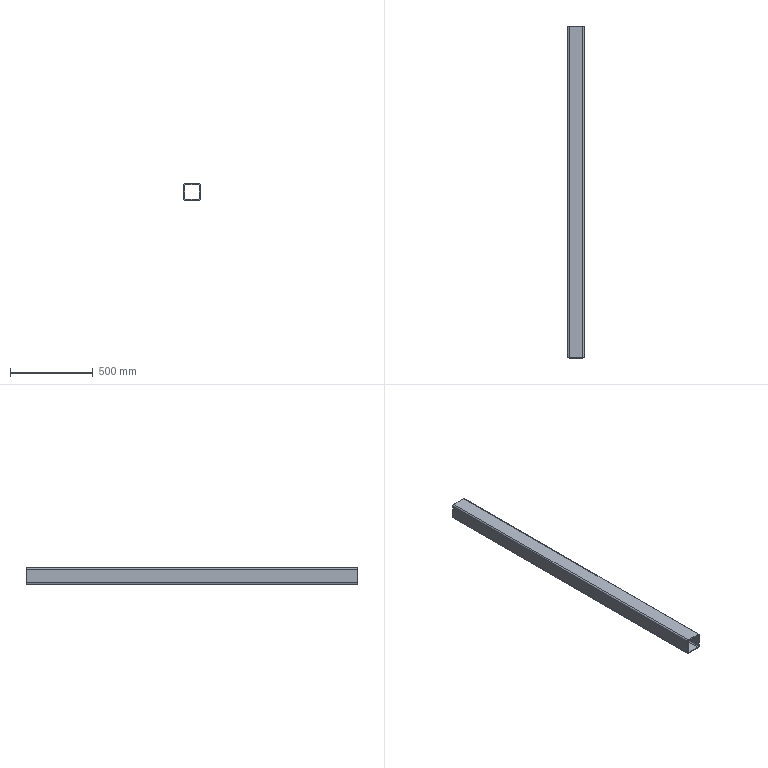Part | SolidWorks | features Extrusion 1 | 1 solid | 18 faces | box 100 x 2000 x 100 mm | volume 4684151 mm3 | plane 10 | cylinder 8 | commonest cylinder face diameters 12.6 x4 15.75 x4
STEP:
#1=CARTESIAN_POINT('',(100.,1000.,-90.6));
#2=VERTEX_POINT('',#1);
#3=CARTESIAN_POINT('',(92.125,1000.,-98.475));
#4=VERTEX_POINT('',#3);
#5=CARTESIAN_POINT('',(92.125,1000.,-90.6));
#6=DIRECTION('',(0.,1.,0.));
#7=DIRECTION('',(0.,0.,1.));
#8=AXIS2_PLACEMENT_3D('',#5,#6,#7);
#9=CIRCLE('',#8,7.875);
#10=EDGE_CURVE('',#2,#4,#9,.T.);
#11=ORIENTED_EDGE('',*,*,#10,.T.);
#12=CARTESIAN_POINT('',(7.875,1000.,-98.475));
#13=VERTEX_POINT('',#12);
#14=CARTESIAN_POINT('',(92.125,1000.,-98.475));
#15=DIRECTION('',(-1.,0.,0.));
#16=VECTOR('',#15,1000.);
#17=LINE('',#14,#16);
#18=EDGE_CURVE('',#4,#13,#17,.T.);
#19=ORIENTED_EDGE('',*,*,#18,.T.);
#20=CARTESIAN_POINT('',(0.,1000.,-90.6));
#21=VERTEX_POINT('',#20);
#22=CARTESIAN_POINT('',(7.875,1000.,-90.6));
#23=DIRECTION('',(0.,1.,0.));
#24=DIRECTION('',(0.,0.,1.));
#25=AXIS2_PLACEMENT_3D('',#22,#23,#24);
#26=CIRCLE('',#25,7.875);
#27=EDGE_CURVE('',#13,#21,#26,.T.);
#28=ORIENTED_EDGE('',*,*,#27,.T.);
#29=CARTESIAN_POINT('',(0.,1000.,-6.35));
#30=VERTEX_POINT('',#29);
#31=CARTESIAN_POINT('',(0.,1000.,-6.35));
#32=DIRECTION('',(0.,0.,1.));
#33=VECTOR('',#32,1000.);
#34=LINE('',#31,#33);
#35=EDGE_CURVE('',#21,#30,#34,.T.);
#36=ORIENTED_EDGE('',*,*,#35,.T.);
#37=CARTESIAN_POINT('',(7.875,1000.,1.525));
#38=VERTEX_POINT('',#37);
#39=CARTESIAN_POINT('',(7.875,1000.,-6.35));
#40=DIRECTION('',(0.,1.,0.));
#41=DIRECTION('',(0.,0.,1.));
#42=AXIS2_PLACEMENT_3D('',#39,#40,#41);
#43=CIRCLE('',#42,7.875);
#44=EDGE_CURVE('',#30,#38,#43,.T.);
#45=ORIENTED_EDGE('',*,*,#44,.T.);
#46=CARTESIAN_POINT('',(92.125,1000.,1.525));
#47=VERTEX_POINT('',#46);
#48=CARTESIAN_POINT('',(7.875,1000.,1.525));
#49=DIRECTION('',(1.,0.,0.));
#50=VECTOR('',#49,1000.);
#51=LINE('',#48,#50);
#52=EDGE_CURVE('',#38,#47,#51,.T.);
#53=ORIENTED_EDGE('',*,*,#52,.T.);
#54=CARTESIAN_POINT('',(100.,1000.,-6.35));
#55=VERTEX_POINT('',#54);
#56=CARTESIAN_POINT('',(92.125,1000.,-6.35));
#57=DIRECTION('',(0.,1.,0.));
#58=DIRECTION('',(0.,0.,1.));
#59=AXIS2_PLACEMENT_3D('',#56,#57,#58);
#60=CIRCLE('',#59,7.875);
#61=EDGE_CURVE('',#47,#55,#60,.T.);
#62=ORIENTED_EDGE('',*,*,#61,.T.);
#63=CARTESIAN_POINT('',(100.,1000.,-90.6));
#64=DIRECTION('',(0.,0.,-1.));
#65=VECTOR('',#64,1000.);
#66=LINE('',#63,#65);
#67=EDGE_CURVE('',#55,#2,#66,.T.);
#68=ORIENTED_EDGE('',*,*,#67,.T.);
#69=EDGE_LOOP('',(#11,#19,#28,#36,#45,#53,#62,#68));
#70=FACE_OUTER_BOUND('',#69,.T.);
#71=CARTESIAN_POINT('',(6.3,1000.,-85.875));
#72=VERTEX_POINT('',#71);
#73=CARTESIAN_POINT('',(6.3,1000.,-11.075));
#74=VERTEX_POINT('',#73);
#75=CARTESIAN_POINT('',(6.3,1000.,-11.075));
#76=DIRECTION('',(0.,0.,1.));
#77=VECTOR('',#76,1000.);
#78=LINE('',#75,#77);
#79=EDGE_CURVE('',#72,#74,#78,.T.);
#80=ORIENTED_EDGE('',*,*,#79,.F.);
#81=CARTESIAN_POINT('',(12.6,1000.,-92.175));
#82=VERTEX_POINT('',#81);
#83=CARTESIAN_POINT('',(12.6,1000.,-85.875));
#84=DIRECTION('',(0.,1.,0.));
#85=DIRECTION('',(0.,0.,1.));
#86=AXIS2_PLACEMENT_3D('',#83,#84,#85);
#87=CIRCLE('',#86,6.3);
#88=EDGE_CURVE('',#82,#72,#87,.T.);
#89=ORIENTED_EDGE('',*,*,#88,.F.);
#90=CARTESIAN_POINT('',(87.4,1000.,-92.175));
#91=VERTEX_POINT('',#90);
#92=CARTESIAN_POINT('',(87.4,1000.,-92.175));
#93=DIRECTION('',(-1.,0.,0.));
#94=VECTOR('',#93,1000.);
#95=LINE('',#92,#94);
#96=EDGE_CURVE('',#91,#82,#95,.T.);
#97=ORIENTED_EDGE('',*,*,#96,.F.);
#98=CARTESIAN_POINT('',(93.7,1000.,-85.875));
#99=VERTEX_POINT('',#98);
#100=CARTESIAN_POINT('',(87.4,1000.,-85.875));
#101=DIRECTION('',(0.,1.,0.));
#102=DIRECTION('',(0.,0.,1.));
#103=AXIS2_PLACEMENT_3D('',#100,#101,#102);
#104=CIRCLE('',#103,6.3);
#105=EDGE_CURVE('',#99,#91,#104,.T.);
#106=ORIENTED_EDGE('',*,*,#105,.F.);
#107=CARTESIAN_POINT('',(93.7,1000.,-11.075));
#108=VERTEX_POINT('',#107);
#109=CARTESIAN_POINT('',(93.7,1000.,-85.875));
#110=DIRECTION('',(0.,0.,-1.));
#111=VECTOR('',#110,1000.);
#112=LINE('',#109,#111);
#113=EDGE_CURVE('',#108,#99,#112,.T.);
#114=ORIENTED_EDGE('',*,*,#113,.F.);
#115=CARTESIAN_POINT('',(87.4,1000.,-4.775));
#116=VERTEX_POINT('',#115);
#117=CARTESIAN_POINT('',(87.4,1000.,-11.075));
#118=DIRECTION('',(0.,1.,0.));
#119=DIRECTION('',(0.,0.,1.));
#120=AXIS2_PLACEMENT_3D('',#117,#118,#119);
#121=CIRCLE('',#120,6.3);
#122=EDGE_CURVE('',#116,#108,#121,.T.);
#123=ORIENTED_EDGE('',*,*,#122,.F.);
#124=CARTESIAN_POINT('',(12.6,1000.,-4.775));
#125=VERTEX_POINT('',#124);
#126=CARTESIAN_POINT('',(12.6,1000.,-4.775));
#127=DIRECTION('',(1.,0.,0.));
#128=VECTOR('',#127,1000.);
#129=LINE('',#126,#128);
#130=EDGE_CURVE('',#125,#116,#129,.T.);
#131=ORIENTED_EDGE('',*,*,#130,.F.);
#132=CARTESIAN_POINT('',(12.6,1000.,-11.075));
#133=DIRECTION('',(0.,1.,0.));
#134=DIRECTION('',(0.,0.,1.));
#135=AXIS2_PLACEMENT_3D('',#132,#133,#134);
#136=CIRCLE('',#135,6.3);
#137=EDGE_CURVE('',#74,#125,#136,.T.);
#138=ORIENTED_EDGE('',*,*,#137,.F.);
#139=EDGE_LOOP('',(#80,#89,#97,#106,#114,#123,#131,#138));
#140=FACE_BOUND('',#139,.T.);
#141=CARTESIAN_POINT('',(92.125,1000.,-90.6));
#142=DIRECTION('',(0.,1.,0.));
#143=DIRECTION('',(0.,0.,1.));
#144=AXIS2_PLACEMENT_3D('',#141,#142,#143);
#145=PLANE('',#144);
#146=ADVANCED_FACE('',(#70,#140),#145,.T.);
#147=CARTESIAN_POINT('',(100.,-1000.,-90.6));
#148=VERTEX_POINT('',#147);
#149=CARTESIAN_POINT('',(92.125,-1000.,-98.475));
#150=VERTEX_POINT('',#149);
#151=CARTESIAN_POINT('',(92.125,-1000.,-90.6));
#152=DIRECTION('',(0.,1.,0.));
#153=DIRECTION('',(0.,0.,1.));
#154=AXIS2_PLACEMENT_3D('',#151,#152,#153);
#155=CIRCLE('',#154,7.875);
#156=EDGE_CURVE('',#148,#150,#155,.T.);
#157=ORIENTED_EDGE('',*,*,#156,.F.);
#158=CARTESIAN_POINT('',(100.,-1000.,-6.35));
#159=VERTEX_POINT('',#158);
#160=CARTESIAN_POINT('',(100.,-1000.,-90.6));
#161=DIRECTION('',(0.,0.,-1.));
#162=VECTOR('',#161,1000.);
#163=LINE('',#160,#162);
#164=EDGE_CURVE('',#159,#148,#163,.T.);
#165=ORIENTED_EDGE('',*,*,#164,.F.);
#166=CARTESIAN_POINT('',(92.125,-1000.,1.525));
#167=VERTEX_POINT('',#166);
#168=CARTESIAN_POINT('',(92.125,-1000.,-6.35));
#169=DIRECTION('',(0.,1.,0.));
#170=DIRECTION('',(0.,0.,1.));
#171=AXIS2_PLACEMENT_3D('',#168,#169,#170);
#172=CIRCLE('',#171,7.875);
#173=EDGE_CURVE('',#167,#159,#172,.T.);
#174=ORIENTED_EDGE('',*,*,#173,.F.);
#175=CARTESIAN_POINT('',(7.875,-1000.,1.525));
#176=VERTEX_POINT('',#175);
#177=CARTESIAN_POINT('',(7.875,-1000.,1.525));
#178=DIRECTION('',(1.,0.,0.));
#179=VECTOR('',#178,1000.);
#180=LINE('',#177,#179);
#181=EDGE_CURVE('',#176,#167,#180,.T.);
#182=ORIENTED_EDGE('',*,*,#181,.F.);
#183=CARTESIAN_POINT('',(0.,-1000.,-6.35));
#184=VERTEX_POINT('',#183);
#185=CARTESIAN_POINT('',(7.875,-1000.,-6.35));
#186=DIRECTION('',(0.,1.,0.));
#187=DIRECTION('',(0.,0.,1.));
#188=AXIS2_PLACEMENT_3D('',#185,#186,#187);
#189=CIRCLE('',#188,7.875);
#190=EDGE_CURVE('',#184,#176,#189,.T.);
#191=ORIENTED_EDGE('',*,*,#190,.F.);
#192=CARTESIAN_POINT('',(0.,-1000.,-90.6));
#193=VERTEX_POINT('',#192);
#194=CARTESIAN_POINT('',(0.,-1000.,-6.35));
#195=DIRECTION('',(0.,0.,1.));
#196=VECTOR('',#195,1000.);
#197=LINE('',#194,#196);
#198=EDGE_CURVE('',#193,#184,#197,.T.);
#199=ORIENTED_EDGE('',*,*,#198,.F.);
#200=CARTESIAN_POINT('',(7.875,-1000.,-98.475));
#201=VERTEX_POINT('',#200);
#202=CARTESIAN_POINT('',(7.875,-1000.,-90.6));
#203=DIRECTION('',(0.,1.,0.));
#204=DIRECTION('',(0.,0.,1.));
#205=AXIS2_PLACEMENT_3D('',#202,#203,#204);
#206=CIRCLE('',#205,7.875);
#207=EDGE_CURVE('',#201,#193,#206,.T.);
#208=ORIENTED_EDGE('',*,*,#207,.F.);
#209=CARTESIAN_POINT('',(92.125,-1000.,-98.475));
#210=DIRECTION('',(-1.,0.,0.));
#211=VECTOR('',#210,1000.);
#212=LINE('',#209,#211);
#213=EDGE_CURVE('',#150,#201,#212,.T.);
#214=ORIENTED_EDGE('',*,*,#213,.F.);
#215=EDGE_LOOP('',(#157,#165,#174,#182,#191,#199,#208,#214));
#216=FACE_OUTER_BOUND('',#215,.T.);
#217=CARTESIAN_POINT('',(12.6,-1000.,-92.175));
#218=VERTEX_POINT('',#217);
#219=CARTESIAN_POINT('',(6.3,-1000.,-85.875));
#220=VERTEX_POINT('',#219);
#221=CARTESIAN_POINT('',(12.6,-1000.,-85.875));
#222=DIRECTION('',(0.,1.,0.));
#223=DIRECTION('',(0.,0.,1.));
#224=AXIS2_PLACEMENT_3D('',#221,#222,#223);
#225=CIRCLE('',#224,6.3);
#226=EDGE_CURVE('',#218,#220,#225,.T.);
#227=ORIENTED_EDGE('',*,*,#226,.T.);
#228=CARTESIAN_POINT('',(6.3,-1000.,-11.075));
#229=VERTEX_POINT('',#228);
#230=CARTESIAN_POINT('',(6.3,-1000.,-11.075));
#231=DIRECTION('',(0.,0.,1.));
#232=VECTOR('',#231,1000.);
#233=LINE('',#230,#232);
#234=EDGE_CURVE('',#220,#229,#233,.T.);
#235=ORIENTED_EDGE('',*,*,#234,.T.);
#236=CARTESIAN_POINT('',(12.6,-1000.,-4.775));
#237=VERTEX_POINT('',#236);
#238=CARTESIAN_POINT('',(12.6,-1000.,-11.075));
#239=DIRECTION('',(0.,1.,0.));
#240=DIRECTION('',(0.,0.,1.));
#241=AXIS2_PLACEMENT_3D('',#238,#239,#240);
#242=CIRCLE('',#241,6.3);
#243=EDGE_CURVE('',#229,#237,#242,.T.);
#244=ORIENTED_EDGE('',*,*,#243,.T.);
#245=CARTESIAN_POINT('',(87.4,-1000.,-4.775));
#246=VERTEX_POINT('',#245);
#247=CARTESIAN_POINT('',(12.6,-1000.,-4.775));
#248=DIRECTION('',(1.,0.,0.));
#249=VECTOR('',#248,1000.);
#250=LINE('',#247,#249);
#251=EDGE_CURVE('',#237,#246,#250,.T.);
#252=ORIENTED_EDGE('',*,*,#251,.T.);
#253=CARTESIAN_POINT('',(93.7,-1000.,-11.075));
#254=VERTEX_POINT('',#253);
#255=CARTESIAN_POINT('',(87.4,-1000.,-11.075));
#256=DIRECTION('',(0.,1.,0.));
#257=DIRECTION('',(0.,0.,1.));
#258=AXIS2_PLACEMENT_3D('',#255,#256,#257);
#259=CIRCLE('',#258,6.3);
#260=EDGE_CURVE('',#246,#254,#259,.T.);
#261=ORIENTED_EDGE('',*,*,#260,.T.);
#262=CARTESIAN_POINT('',(93.7,-1000.,-85.875));
#263=VERTEX_POINT('',#262);
#264=CARTESIAN_POINT('',(93.7,-1000.,-85.875));
#265=DIRECTION('',(0.,0.,-1.));
#266=VECTOR('',#265,1000.);
#267=LINE('',#264,#266);
#268=EDGE_CURVE('',#254,#263,#267,.T.);
#269=ORIENTED_EDGE('',*,*,#268,.T.);
#270=CARTESIAN_POINT('',(87.4,-1000.,-92.175));
#271=VERTEX_POINT('',#270);
#272=CARTESIAN_POINT('',(87.4,-1000.,-85.875));
#273=DIRECTION('',(0.,1.,0.));
#274=DIRECTION('',(0.,0.,1.));
#275=AXIS2_PLACEMENT_3D('',#272,#273,#274);
#276=CIRCLE('',#275,6.3);
#277=EDGE_CURVE('',#263,#271,#276,.T.);
#278=ORIENTED_EDGE('',*,*,#277,.T.);
#279=CARTESIAN_POINT('',(87.4,-1000.,-92.175));
#280=DIRECTION('',(-1.,0.,0.));
#281=VECTOR('',#280,1000.);
#282=LINE('',#279,#281);
#283=EDGE_CURVE('',#271,#218,#282,.T.);
#284=ORIENTED_EDGE('',*,*,#283,.T.);
#285=EDGE_LOOP('',(#227,#235,#244,#252,#261,#269,#278,#284));
#286=FACE_BOUND('',#285,.T.);
#287=CARTESIAN_POINT('',(92.125,-1000.,-90.6));
#288=DIRECTION('',(0.,1.,0.));
#289=DIRECTION('',(0.,0.,1.));
#290=AXIS2_PLACEMENT_3D('',#287,#288,#289);
#291=PLANE('',#290);
#292=ADVANCED_FACE('',(#216,#286),#291,.F.);
#293=ORIENTED_EDGE('',*,*,#156,.T.);
#294=CARTESIAN_POINT('',(92.125,1000.,-98.475));
#295=DIRECTION('',(0.,-1.,0.));
#296=VECTOR('',#295,1000.);
#297=LINE('',#294,#296);
#298=EDGE_CURVE('',#4,#150,#297,.T.);
#299=ORIENTED_EDGE('',*,*,#298,.F.);
#300=ORIENTED_EDGE('',*,*,#10,.F.);
#301=CARTESIAN_POINT('',(100.,1000.,-90.6));
#302=DIRECTION('',(0.,-1.,0.));
#303=VECTOR('',#302,1000.);
#304=LINE('',#301,#303);
#305=EDGE_CURVE('',#2,#148,#304,.T.);
#306=ORIENTED_EDGE('',*,*,#305,.T.);
#307=EDGE_LOOP('',(#293,#299,#300,#306));
#308=FACE_OUTER_BOUND('',#307,.T.);
#309=CARTESIAN_POINT('',(92.125,1000.,-90.6));
#310=DIRECTION('',(0.,-1.,0.));
#311=DIRECTION('',(0.,0.,-1.));
#312=AXIS2_PLACEMENT_3D('',#309,#310,#311);
#313=CYLINDRICAL_SURFACE('',#312,7.875);
#314=ADVANCED_FACE('',(#308),#313,.T.);
#315=ORIENTED_EDGE('',*,*,#213,.T.);
#316=CARTESIAN_POINT('',(7.875,1000.,-98.475));
#317=DIRECTION('',(0.,-1.,0.));
#318=VECTOR('',#317,1000.);
#319=LINE('',#316,#318);
#320=EDGE_CURVE('',#13,#201,#319,.T.);
#321=ORIENTED_EDGE('',*,*,#320,.F.);
#322=ORIENTED_EDGE('',*,*,#18,.F.);
#323=ORIENTED_EDGE('',*,*,#298,.T.);
#324=EDGE_LOOP('',(#315,#321,#322,#323));
#325=FACE_OUTER_BOUND('',#324,.T.);
#326=CARTESIAN_POINT('',(92.125,1000.,-98.475));
#327=DIRECTION('',(0.,0.,1.));
#328=DIRECTION('',(1.,0.,0.));
#329=AXIS2_PLACEMENT_3D('',#326,#327,#328);
#330=PLANE('',#329);
#331=ADVANCED_FACE('',(#325),#330,.F.);
#332=ORIENTED_EDGE('',*,*,#207,.T.);
#333=CARTESIAN_POINT('',(0.,1000.,-90.6));
#334=DIRECTION('',(0.,-1.,0.));
#335=VECTOR('',#334,1000.);
#336=LINE('',#333,#335);
#337=EDGE_CURVE('',#21,#193,#336,.T.);
#338=ORIENTED_EDGE('',*,*,#337,.F.);
#339=ORIENTED_EDGE('',*,*,#27,.F.);
#340=ORIENTED_EDGE('',*,*,#320,.T.);
#341=EDGE_LOOP('',(#332,#338,#339,#340));
#342=FACE_OUTER_BOUND('',#341,.T.);
#343=CARTESIAN_POINT('',(7.875,1000.,-90.6));
#344=DIRECTION('',(0.,-1.,0.));
#345=DIRECTION('',(0.,0.,-1.));
#346=AXIS2_PLACEMENT_3D('',#343,#344,#345);
#347=CYLINDRICAL_SURFACE('',#346,7.875);
#348=ADVANCED_FACE('',(#342),#347,.T.);
#349=ORIENTED_EDGE('',*,*,#198,.T.);
#350=CARTESIAN_POINT('',(0.,1000.,-6.35));
#351=DIRECTION('',(0.,-1.,0.));
#352=VECTOR('',#351,1000.);
#353=LINE('',#350,#352);
#354=EDGE_CURVE('',#30,#184,#353,.T.);
#355=ORIENTED_EDGE('',*,*,#354,.F.);
#356=ORIENTED_EDGE('',*,*,#35,.F.);
#357=ORIENTED_EDGE('',*,*,#337,.T.);
#358=EDGE_LOOP('',(#349,#355,#356,#357));
#359=FACE_OUTER_BOUND('',#358,.T.);
#360=CARTESIAN_POINT('',(0.,1000.,-6.35));
#361=DIRECTION('',(1.,0.,0.));
#362=DIRECTION('',(0.,0.,-1.));
#363=AXIS2_PLACEMENT_3D('',#360,#361,#362);
#364=PLANE('',#363);
#365=ADVANCED_FACE('',(#359),#364,.F.);
#366=ORIENTED_EDGE('',*,*,#190,.T.);
#367=CARTESIAN_POINT('',(7.875,1000.,1.525));
#368=DIRECTION('',(0.,-1.,0.));
#369=VECTOR('',#368,1000.);
#370=LINE('',#367,#369);
#371=EDGE_CURVE('',#38,#176,#370,.T.);
#372=ORIENTED_EDGE('',*,*,#371,.F.);
#373=ORIENTED_EDGE('',*,*,#44,.F.);
#374=ORIENTED_EDGE('',*,*,#354,.T.);
#375=EDGE_LOOP('',(#366,#372,#373,#374));
#376=FACE_OUTER_BOUND('',#375,.T.);
#377=CARTESIAN_POINT('',(7.875,1000.,-6.35));
#378=DIRECTION('',(0.,-1.,0.));
#379=DIRECTION('',(0.,0.,-1.));
#380=AXIS2_PLACEMENT_3D('',#377,#378,#379);
#381=CYLINDRICAL_SURFACE('',#380,7.875);
#382=ADVANCED_FACE('',(#376),#381,.T.);
#383=ORIENTED_EDGE('',*,*,#181,.T.);
#384=CARTESIAN_POINT('',(92.125,1000.,1.525));
#385=DIRECTION('',(0.,-1.,0.));
#386=VECTOR('',#385,1000.);
#387=LINE('',#384,#386);
#388=EDGE_CURVE('',#47,#167,#387,.T.);
#389=ORIENTED_EDGE('',*,*,#388,.F.);
#390=ORIENTED_EDGE('',*,*,#52,.F.);
#391=ORIENTED_EDGE('',*,*,#371,.T.);
#392=EDGE_LOOP('',(#383,#389,#390,#391));
#393=FACE_OUTER_BOUND('',#392,.T.);
#394=CARTESIAN_POINT('',(7.875,1000.,1.525));
#395=DIRECTION('',(0.,0.,-1.));
#396=DIRECTION('',(-1.,0.,0.));
#397=AXIS2_PLACEMENT_3D('',#394,#395,#396);
#398=PLANE('',#397);
#399=ADVANCED_FACE('',(#393),#398,.F.);
#400=ORIENTED_EDGE('',*,*,#173,.T.);
#401=CARTESIAN_POINT('',(100.,1000.,-6.35));
#402=DIRECTION('',(0.,-1.,0.));
#403=VECTOR('',#402,1000.);
#404=LINE('',#401,#403);
#405=EDGE_CURVE('',#55,#159,#404,.T.);
#406=ORIENTED_EDGE('',*,*,#405,.F.);
#407=ORIENTED_EDGE('',*,*,#61,.F.);
#408=ORIENTED_EDGE('',*,*,#388,.T.);
#409=EDGE_LOOP('',(#400,#406,#407,#408));
#410=FACE_OUTER_BOUND('',#409,.T.);
#411=CARTESIAN_POINT('',(92.125,1000.,-6.35));
#412=DIRECTION('',(0.,-1.,0.));
#413=DIRECTION('',(0.,0.,-1.));
#414=AXIS2_PLACEMENT_3D('',#411,#412,#413);
#415=CYLINDRICAL_SURFACE('',#414,7.875);
#416=ADVANCED_FACE('',(#410),#415,.T.);
#417=ORIENTED_EDGE('',*,*,#164,.T.);
#418=ORIENTED_EDGE('',*,*,#305,.F.);
#419=ORIENTED_EDGE('',*,*,#67,.F.);
#420=ORIENTED_EDGE('',*,*,#405,.T.);
#421=EDGE_LOOP('',(#417,#418,#419,#420));
#422=FACE_OUTER_BOUND('',#421,.T.);
#423=CARTESIAN_POINT('',(100.,1000.,-90.6));
#424=DIRECTION('',(-1.,0.,0.));
#425=DIRECTION('',(0.,0.,1.));
#426=AXIS2_PLACEMENT_3D('',#423,#424,#425);
#427=PLANE('',#426);
#428=ADVANCED_FACE('',(#422),#427,.F.);
#429=ORIENTED_EDGE('',*,*,#226,.F.);
#430=CARTESIAN_POINT('',(12.6,1000.,-92.175));
#431=DIRECTION('',(0.,-1.,0.));
#432=VECTOR('',#431,1000.);
#433=LINE('',#430,#432);
#434=EDGE_CURVE('',#82,#218,#433,.T.);
#435=ORIENTED_EDGE('',*,*,#434,.F.);
#436=ORIENTED_EDGE('',*,*,#88,.T.);
#437=CARTESIAN_POINT('',(6.3,1000.,-85.875));
#438=DIRECTION('',(0.,-1.,0.));
#439=VECTOR('',#438,1000.);
#440=LINE('',#437,#439);
#441=EDGE_CURVE('',#72,#220,#440,.T.);
#442=ORIENTED_EDGE('',*,*,#441,.T.);
#443=EDGE_LOOP('',(#429,#435,#436,#442));
#444=FACE_OUTER_BOUND('',#443,.T.);
#445=CARTESIAN_POINT('',(12.6,1000.,-85.875));
#446=DIRECTION('',(0.,-1.,0.));
#447=DIRECTION('',(0.,0.,-1.));
#448=AXIS2_PLACEMENT_3D('',#445,#446,#447);
#449=CYLINDRICAL_SURFACE('',#448,6.3);
#450=ADVANCED_FACE('',(#444),#449,.F.);
#451=ORIENTED_EDGE('',*,*,#234,.F.);
#452=ORIENTED_EDGE('',*,*,#441,.F.);
#453=ORIENTED_EDGE('',*,*,#79,.T.);
#454=CARTESIAN_POINT('',(6.3,1000.,-11.075));
#455=DIRECTION('',(0.,-1.,0.));
#456=VECTOR('',#455,1000.);
#457=LINE('',#454,#456);
#458=EDGE_CURVE('',#74,#229,#457,.T.);
#459=ORIENTED_EDGE('',*,*,#458,.T.);
#460=EDGE_LOOP('',(#451,#452,#453,#459));
#461=FACE_OUTER_BOUND('',#460,.T.);
#462=CARTESIAN_POINT('',(6.3,1000.,-11.075));
#463=DIRECTION('',(1.,0.,0.));
#464=DIRECTION('',(0.,0.,-1.));
#465=AXIS2_PLACEMENT_3D('',#462,#463,#464);
#466=PLANE('',#465);
#467=ADVANCED_FACE('',(#461),#466,.T.);
#468=ORIENTED_EDGE('',*,*,#243,.F.);
#469=ORIENTED_EDGE('',*,*,#458,.F.);
#470=ORIENTED_EDGE('',*,*,#137,.T.);
#471=CARTESIAN_POINT('',(12.6,1000.,-4.775));
#472=DIRECTION('',(0.,-1.,0.));
#473=VECTOR('',#472,1000.);
#474=LINE('',#471,#473);
#475=EDGE_CURVE('',#125,#237,#474,.T.);
#476=ORIENTED_EDGE('',*,*,#475,.T.);
#477=EDGE_LOOP('',(#468,#469,#470,#476));
#478=FACE_OUTER_BOUND('',#477,.T.);
#479=CARTESIAN_POINT('',(12.6,1000.,-11.075));
#480=DIRECTION('',(0.,-1.,0.));
#481=DIRECTION('',(0.,0.,-1.));
#482=AXIS2_PLACEMENT_3D('',#479,#480,#481);
#483=CYLINDRICAL_SURFACE('',#482,6.3);
#484=ADVANCED_FACE('',(#478),#483,.F.);
#485=ORIENTED_EDGE('',*,*,#251,.F.);
#486=ORIENTED_EDGE('',*,*,#475,.F.);
#487=ORIENTED_EDGE('',*,*,#130,.T.);
#488=CARTESIAN_POINT('',(87.4,1000.,-4.775));
#489=DIRECTION('',(0.,-1.,0.));
#490=VECTOR('',#489,1000.);
#491=LINE('',#488,#490);
#492=EDGE_CURVE('',#116,#246,#491,.T.);
#493=ORIENTED_EDGE('',*,*,#492,.T.);
#494=EDGE_LOOP('',(#485,#486,#487,#493));
#495=FACE_OUTER_BOUND('',#494,.T.);
#496=CARTESIAN_POINT('',(12.6,1000.,-4.775));
#497=DIRECTION('',(0.,0.,-1.));
#498=DIRECTION('',(-1.,0.,0.));
#499=AXIS2_PLACEMENT_3D('',#496,#497,#498);
#500=PLANE('',#499);
#501=ADVANCED_FACE('',(#495),#500,.T.);
#502=ORIENTED_EDGE('',*,*,#260,.F.);
#503=ORIENTED_EDGE('',*,*,#492,.F.);
#504=ORIENTED_EDGE('',*,*,#122,.T.);
#505=CARTESIAN_POINT('',(93.7,1000.,-11.075));
#506=DIRECTION('',(0.,-1.,0.));
#507=VECTOR('',#506,1000.);
#508=LINE('',#505,#507);
#509=EDGE_CURVE('',#108,#254,#508,.T.);
#510=ORIENTED_EDGE('',*,*,#509,.T.);
#511=EDGE_LOOP('',(#502,#503,#504,#510));
#512=FACE_OUTER_BOUND('',#511,.T.);
#513=CARTESIAN_POINT('',(87.4,1000.,-11.075));
#514=DIRECTION('',(0.,-1.,0.));
#515=DIRECTION('',(0.,0.,-1.));
#516=AXIS2_PLACEMENT_3D('',#513,#514,#515);
#517=CYLINDRICAL_SURFACE('',#516,6.3);
#518=ADVANCED_FACE('',(#512),#517,.F.);
#519=ORIENTED_EDGE('',*,*,#268,.F.);
#520=ORIENTED_EDGE('',*,*,#509,.F.);
#521=ORIENTED_EDGE('',*,*,#113,.T.);
#522=CARTESIAN_POINT('',(93.7,1000.,-85.875));
#523=DIRECTION('',(0.,-1.,0.));
#524=VECTOR('',#523,1000.);
#525=LINE('',#522,#524);
#526=EDGE_CURVE('',#99,#263,#525,.T.);
#527=ORIENTED_EDGE('',*,*,#526,.T.);
#528=EDGE_LOOP('',(#519,#520,#521,#527));
#529=FACE_OUTER_BOUND('',#528,.T.);
#530=CARTESIAN_POINT('',(93.7,1000.,-85.875));
#531=DIRECTION('',(-1.,0.,0.));
#532=DIRECTION('',(0.,0.,1.));
#533=AXIS2_PLACEMENT_3D('',#530,#531,#532);
#534=PLANE('',#533);
#535=ADVANCED_FACE('',(#529),#534,.T.);
#536=ORIENTED_EDGE('',*,*,#277,.F.);
#537=ORIENTED_EDGE('',*,*,#526,.F.);
#538=ORIENTED_EDGE('',*,*,#105,.T.);
#539=CARTESIAN_POINT('',(87.4,1000.,-92.175));
#540=DIRECTION('',(0.,-1.,0.));
#541=VECTOR('',#540,1000.);
#542=LINE('',#539,#541);
#543=EDGE_CURVE('',#91,#271,#542,.T.);
#544=ORIENTED_EDGE('',*,*,#543,.T.);
#545=EDGE_LOOP('',(#536,#537,#538,#544));
#546=FACE_OUTER_BOUND('',#545,.T.);
#547=CARTESIAN_POINT('',(87.4,1000.,-85.875));
#548=DIRECTION('',(0.,-1.,0.));
#549=DIRECTION('',(0.,0.,-1.));
#550=AXIS2_PLACEMENT_3D('',#547,#548,#549);
#551=CYLINDRICAL_SURFACE('',#550,6.3);
#552=ADVANCED_FACE('',(#546),#551,.F.);
#553=ORIENTED_EDGE('',*,*,#283,.F.);
#554=ORIENTED_EDGE('',*,*,#543,.F.);
#555=ORIENTED_EDGE('',*,*,#96,.T.);
#556=ORIENTED_EDGE('',*,*,#434,.T.);
#557=EDGE_LOOP('',(#553,#554,#555,#556));
#558=FACE_OUTER_BOUND('',#557,.T.);
#559=CARTESIAN_POINT('',(87.4,1000.,-92.175));
#560=DIRECTION('',(0.,0.,1.));
#561=DIRECTION('',(1.,0.,0.));
#562=AXIS2_PLACEMENT_3D('',#559,#560,#561);
#563=PLANE('',#562);
#564=ADVANCED_FACE('',(#558),#563,.T.);
#565=CLOSED_SHELL('',(#146,#292,#314,#331,#348,#365,#382,#399,#416,#428,#450,#467,#484,#501,#518,#535,#552,#564));
#566=MANIFOLD_SOLID_BREP('',#565);
#567=CARTESIAN_POINT('',(0.,0.,0.));
#568=DIRECTION('',(0.,0.,1.));
#569=DIRECTION('',(1.,0.,0.));
#570=AXIS2_PLACEMENT_3D('',#567,#568,#569);
#571=(LENGTH_UNIT()NAMED_UNIT(*)SI_UNIT(.MILLI.,.METRE.));
#572=UNCERTAINTY_MEASURE_WITH_UNIT(LENGTH_MEASURE(0.00001),#571,'','');
#573=(NAMED_UNIT(*)PLANE_ANGLE_UNIT()SI_UNIT($,.RADIAN.));
#574=(NAMED_UNIT(*)SI_UNIT($,.STERADIAN.)SOLID_ANGLE_UNIT());
#575=(GEOMETRIC_REPRESENTATION_CONTEXT(3)GLOBAL_UNCERTAINTY_ASSIGNED_CONTEXT((#572))GLOBAL_UNIT_ASSIGNED_CONTEXT((#571,#573,#574))REPRESENTATION_CONTEXT('',''));
#576=ADVANCED_BREP_SHAPE_REPRESENTATION('',(#566,#570),#575);